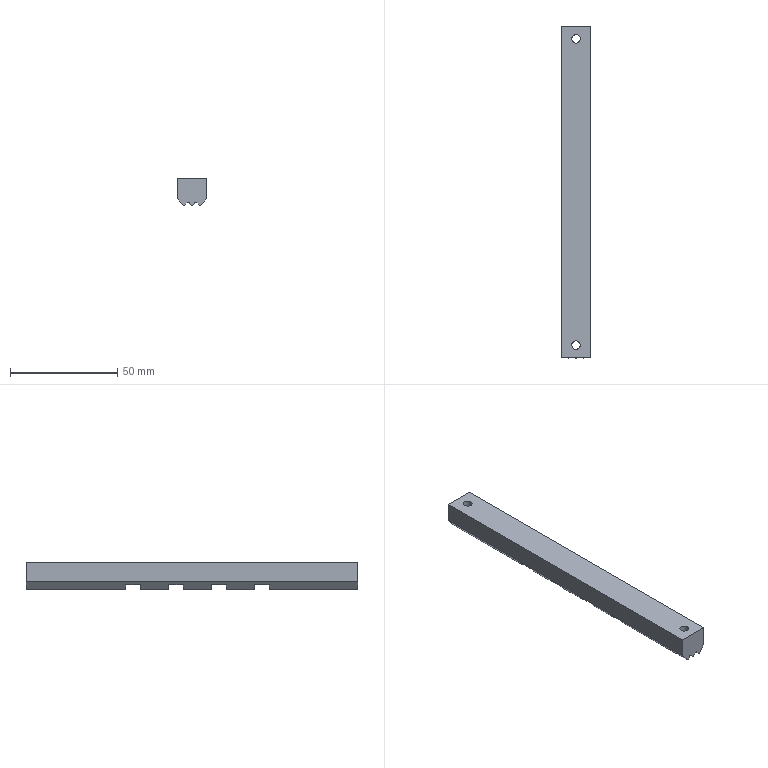Part | STEP file | 200 mesh_id2174 | 1 solid | 106 faces | box 14 x 155 x 12.945 mm | volume 24551 mm3 | plane 60 | cylinder 46 | commonest cylinder face diameters 1.04 x34 1.2 x10 4 x2